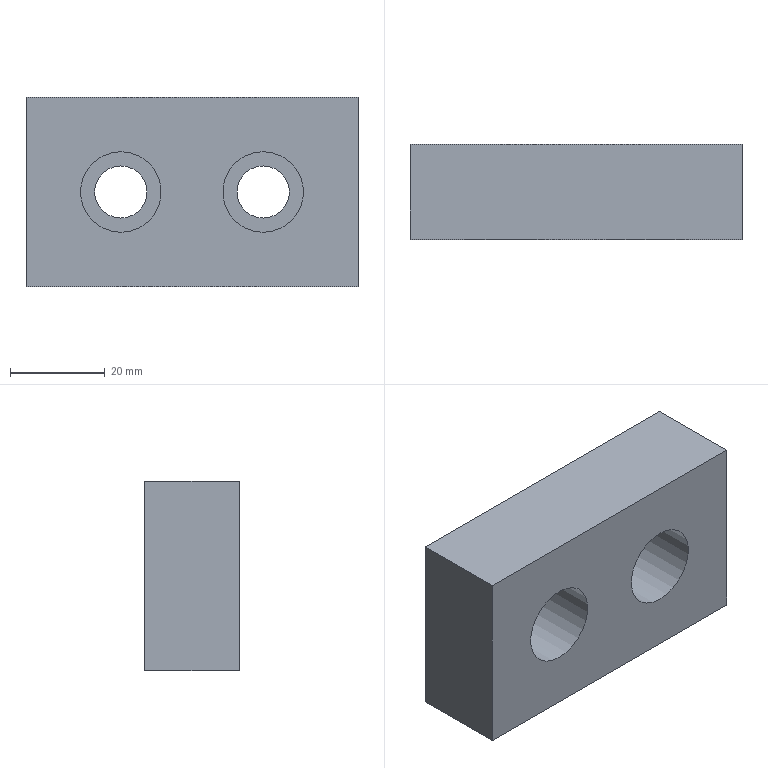Part | NX | features solid 2 | 1 solid | 12 faces | box 70 x 20 x 40 mm | volume 49032 mm3 | plane 8 | cylinder 4 | commonest cylinder face diameters 11 x2 17 x2
STEP:
#1=CARTESIAN_POINT('',(-1202.5,-895.,-295.));
#2=VERTEX_POINT('',#1);
#3=CARTESIAN_POINT('',(-1202.5,-895.,-335.));
#4=VERTEX_POINT('',#3);
#5=CARTESIAN_POINT('',(-1202.5,-895.,-340.));
#6=DIRECTION('',(0.,0.,-1.));
#7=VECTOR('',#6,1000.);
#8=LINE('',#5,#7);
#9=EDGE_CURVE('',#2,#4,#8,.T.);
#10=ORIENTED_EDGE('',*,*,#9,.F.);
#11=CARTESIAN_POINT('',(-1202.5,-875.,-295.));
#12=VERTEX_POINT('',#11);
#13=CARTESIAN_POINT('',(-1202.5,-875.,-295.));
#14=DIRECTION('',(0.,-1.,0.));
#15=VECTOR('',#14,1000.);
#16=LINE('',#13,#15);
#17=EDGE_CURVE('',#12,#2,#16,.T.);
#18=ORIENTED_EDGE('',*,*,#17,.F.);
#19=CARTESIAN_POINT('',(-1202.5,-875.,-335.));
#20=VERTEX_POINT('',#19);
#21=CARTESIAN_POINT('',(-1202.5,-875.,-340.));
#22=DIRECTION('',(0.,0.,-1.));
#23=VECTOR('',#22,1000.);
#24=LINE('',#21,#23);
#25=EDGE_CURVE('',#12,#20,#24,.T.);
#26=ORIENTED_EDGE('',*,*,#25,.T.);
#27=CARTESIAN_POINT('',(-1202.5,-875.,-335.));
#28=DIRECTION('',(0.,-1.,0.));
#29=VECTOR('',#28,1000.);
#30=LINE('',#27,#29);
#31=EDGE_CURVE('',#20,#4,#30,.T.);
#32=ORIENTED_EDGE('',*,*,#31,.T.);
#33=EDGE_LOOP('',(#10,#18,#26,#32));
#34=FACE_BOUND('',#33,.T.);
#35=CARTESIAN_POINT('',(-1202.5,-875.,-340.));
#36=DIRECTION('',(1.,0.,0.));
#37=DIRECTION('',(0.,0.,1.));
#38=AXIS2_PLACEMENT_3D('',#35,#36,#37);
#39=PLANE('',#38);
#40=ADVANCED_FACE('',(#34),#39,.F.);
#41=CARTESIAN_POINT('',(-1132.5,-895.,-295.));
#42=VERTEX_POINT('',#41);
#43=CARTESIAN_POINT('',(77.5,-895.,-295.));
#44=DIRECTION('',(1.,0.,0.));
#45=VECTOR('',#44,1000.);
#46=LINE('',#43,#45);
#47=EDGE_CURVE('',#2,#42,#46,.T.);
#48=ORIENTED_EDGE('',*,*,#47,.T.);
#49=CARTESIAN_POINT('',(-1132.5,-875.,-295.));
#50=VERTEX_POINT('',#49);
#51=CARTESIAN_POINT('',(-1132.5,-875.,-295.));
#52=DIRECTION('',(0.,-1.,0.));
#53=VECTOR('',#52,1000.);
#54=LINE('',#51,#53);
#55=EDGE_CURVE('',#50,#42,#54,.T.);
#56=ORIENTED_EDGE('',*,*,#55,.F.);
#57=CARTESIAN_POINT('',(77.5,-875.,-295.));
#58=DIRECTION('',(1.,0.,0.));
#59=VECTOR('',#58,1000.);
#60=LINE('',#57,#59);
#61=EDGE_CURVE('',#12,#50,#60,.T.);
#62=ORIENTED_EDGE('',*,*,#61,.F.);
#63=ORIENTED_EDGE('',*,*,#17,.T.);
#64=EDGE_LOOP('',(#48,#56,#62,#63));
#65=FACE_BOUND('',#64,.T.);
#66=CARTESIAN_POINT('',(77.5,-875.,-295.));
#67=DIRECTION('',(0.,0.,1.));
#68=DIRECTION('',(-1.,0.,0.));
#69=AXIS2_PLACEMENT_3D('',#66,#67,#68);
#70=PLANE('',#69);
#71=ADVANCED_FACE('',(#65),#70,.T.);
#72=CARTESIAN_POINT('',(-1132.5,-895.,-335.));
#73=VERTEX_POINT('',#72);
#74=CARTESIAN_POINT('',(-1132.5,-895.,-340.));
#75=DIRECTION('',(0.,0.,1.));
#76=VECTOR('',#75,1000.);
#77=LINE('',#74,#76);
#78=EDGE_CURVE('',#73,#42,#77,.T.);
#79=ORIENTED_EDGE('',*,*,#78,.F.);
#80=CARTESIAN_POINT('',(-1132.5,-875.,-335.));
#81=VERTEX_POINT('',#80);
#82=CARTESIAN_POINT('',(-1132.5,-875.,-335.));
#83=DIRECTION('',(0.,-1.,0.));
#84=VECTOR('',#83,1000.);
#85=LINE('',#82,#84);
#86=EDGE_CURVE('',#81,#73,#85,.T.);
#87=ORIENTED_EDGE('',*,*,#86,.F.);
#88=CARTESIAN_POINT('',(-1132.5,-875.,-340.));
#89=DIRECTION('',(0.,0.,1.));
#90=VECTOR('',#89,1000.);
#91=LINE('',#88,#90);
#92=EDGE_CURVE('',#81,#50,#91,.T.);
#93=ORIENTED_EDGE('',*,*,#92,.T.);
#94=ORIENTED_EDGE('',*,*,#55,.T.);
#95=EDGE_LOOP('',(#79,#87,#93,#94));
#96=FACE_BOUND('',#95,.T.);
#97=CARTESIAN_POINT('',(-1132.5,-875.,-340.));
#98=DIRECTION('',(-1.,0.,0.));
#99=DIRECTION('',(0.,0.,-1.));
#100=AXIS2_PLACEMENT_3D('',#97,#98,#99);
#101=PLANE('',#100);
#102=ADVANCED_FACE('',(#96),#101,.F.);
#103=CARTESIAN_POINT('',(77.5,-895.,-335.));
#104=DIRECTION('',(-1.,0.,0.));
#105=VECTOR('',#104,1000.);
#106=LINE('',#103,#105);
#107=EDGE_CURVE('',#73,#4,#106,.T.);
#108=ORIENTED_EDGE('',*,*,#107,.T.);
#109=ORIENTED_EDGE('',*,*,#31,.F.);
#110=CARTESIAN_POINT('',(77.5,-875.,-335.));
#111=DIRECTION('',(-1.,0.,0.));
#112=VECTOR('',#111,1000.);
#113=LINE('',#110,#112);
#114=EDGE_CURVE('',#81,#20,#113,.T.);
#115=ORIENTED_EDGE('',*,*,#114,.F.);
#116=ORIENTED_EDGE('',*,*,#86,.T.);
#117=EDGE_LOOP('',(#108,#109,#115,#116));
#118=FACE_BOUND('',#117,.T.);
#119=CARTESIAN_POINT('',(77.5,-875.,-335.));
#120=DIRECTION('',(0.,0.,-1.));
#121=DIRECTION('',(1.,0.,0.));
#122=AXIS2_PLACEMENT_3D('',#119,#120,#121);
#123=PLANE('',#122);
#124=ADVANCED_FACE('',(#118),#123,.T.);
#125=CARTESIAN_POINT('',(-1182.5,-875.,-309.5));
#126=VERTEX_POINT('',#125);
#127=CARTESIAN_POINT('',(-1182.5,-875.,-315.));
#128=DIRECTION('',(0.,-1.,0.));
#129=DIRECTION('',(0.,0.,1.));
#130=AXIS2_PLACEMENT_3D('',#127,#128,#129);
#131=CIRCLE('',#130,5.5);
#132=EDGE_CURVE('',#126,#126,#131,.T.);
#133=ORIENTED_EDGE('',*,*,#132,.T.);
#134=EDGE_LOOP('',(#133));
#135=FACE_BOUND('',#134,.T.);
#136=CARTESIAN_POINT('',(-1152.5,-875.,-309.5));
#137=VERTEX_POINT('',#136);
#138=CARTESIAN_POINT('',(-1152.5,-875.,-315.));
#139=DIRECTION('',(0.,-1.,0.));
#140=DIRECTION('',(0.,0.,1.));
#141=AXIS2_PLACEMENT_3D('',#138,#139,#140);
#142=CIRCLE('',#141,5.5);
#143=EDGE_CURVE('',#137,#137,#142,.T.);
#144=ORIENTED_EDGE('',*,*,#143,.T.);
#145=EDGE_LOOP('',(#144));
#146=FACE_BOUND('',#145,.T.);
#147=ORIENTED_EDGE('',*,*,#25,.F.);
#148=ORIENTED_EDGE('',*,*,#61,.T.);
#149=ORIENTED_EDGE('',*,*,#92,.F.);
#150=ORIENTED_EDGE('',*,*,#114,.T.);
#151=EDGE_LOOP('',(#147,#148,#149,#150));
#152=FACE_BOUND('',#151,.T.);
#153=CARTESIAN_POINT('',(-1217.5,-875.,-340.));
#154=DIRECTION('',(0.,1.,0.));
#155=DIRECTION('',(1.,0.,0.));
#156=AXIS2_PLACEMENT_3D('',#153,#154,#155);
#157=PLANE('',#156);
#158=ADVANCED_FACE('',(#135,#146,#152),#157,.T.);
#159=CARTESIAN_POINT('',(-1182.5,-895.,-306.5));
#160=VERTEX_POINT('',#159);
#161=CARTESIAN_POINT('',(-1182.5,-895.,-315.));
#162=DIRECTION('',(0.,-1.,0.));
#163=DIRECTION('',(0.,0.,1.));
#164=AXIS2_PLACEMENT_3D('',#161,#162,#163);
#165=CIRCLE('',#164,8.5);
#166=EDGE_CURVE('',#160,#160,#165,.T.);
#167=ORIENTED_EDGE('',*,*,#166,.F.);
#168=EDGE_LOOP('',(#167));
#169=FACE_BOUND('',#168,.T.);
#170=CARTESIAN_POINT('',(-1152.5,-895.,-306.5));
#171=VERTEX_POINT('',#170);
#172=CARTESIAN_POINT('',(-1152.5,-895.,-315.));
#173=DIRECTION('',(0.,-1.,0.));
#174=DIRECTION('',(0.,0.,1.));
#175=AXIS2_PLACEMENT_3D('',#172,#173,#174);
#176=CIRCLE('',#175,8.5);
#177=EDGE_CURVE('',#171,#171,#176,.T.);
#178=ORIENTED_EDGE('',*,*,#177,.F.);
#179=EDGE_LOOP('',(#178));
#180=FACE_BOUND('',#179,.T.);
#181=ORIENTED_EDGE('',*,*,#9,.T.);
#182=ORIENTED_EDGE('',*,*,#107,.F.);
#183=ORIENTED_EDGE('',*,*,#78,.T.);
#184=ORIENTED_EDGE('',*,*,#47,.F.);
#185=EDGE_LOOP('',(#181,#182,#183,#184));
#186=FACE_BOUND('',#185,.T.);
#187=CARTESIAN_POINT('',(-1217.5,-895.,-340.));
#188=DIRECTION('',(0.,1.,0.));
#189=DIRECTION('',(1.,0.,0.));
#190=AXIS2_PLACEMENT_3D('',#187,#188,#189);
#191=PLANE('',#190);
#192=ADVANCED_FACE('',(#169,#180,#186),#191,.F.);
#193=ORIENTED_EDGE('',*,*,#143,.F.);
#194=EDGE_LOOP('',(#193));
#195=FACE_BOUND('',#194,.T.);
#196=CARTESIAN_POINT('',(-1152.5,-883.,-309.5));
#197=VERTEX_POINT('',#196);
#198=CARTESIAN_POINT('',(-1152.5,-883.,-315.));
#199=DIRECTION('',(0.,-1.,0.));
#200=DIRECTION('',(0.,0.,1.));
#201=AXIS2_PLACEMENT_3D('',#198,#199,#200);
#202=CIRCLE('',#201,5.5);
#203=EDGE_CURVE('',#197,#197,#202,.T.);
#204=ORIENTED_EDGE('',*,*,#203,.T.);
#205=EDGE_LOOP('',(#204));
#206=FACE_BOUND('',#205,.T.);
#207=CARTESIAN_POINT('',(-1152.5,-845.,-315.));
#208=DIRECTION('',(0.,1.,0.));
#209=DIRECTION('',(0.,0.,1.));
#210=AXIS2_PLACEMENT_3D('',#207,#208,#209);
#211=CYLINDRICAL_SURFACE('',#210,5.5);
#212=ADVANCED_FACE('',(#195,#206),#211,.F.);
#213=ORIENTED_EDGE('',*,*,#203,.F.);
#214=EDGE_LOOP('',(#213));
#215=FACE_BOUND('',#214,.T.);
#216=CARTESIAN_POINT('',(-1152.5,-883.,-306.5));
#217=VERTEX_POINT('',#216);
#218=CARTESIAN_POINT('',(-1152.5,-883.,-315.));
#219=DIRECTION('',(0.,-1.,0.));
#220=DIRECTION('',(0.,0.,1.));
#221=AXIS2_PLACEMENT_3D('',#218,#219,#220);
#222=CIRCLE('',#221,8.5);
#223=EDGE_CURVE('',#217,#217,#222,.T.);
#224=ORIENTED_EDGE('',*,*,#223,.T.);
#225=EDGE_LOOP('',(#224));
#226=FACE_BOUND('',#225,.T.);
#227=CARTESIAN_POINT('',(-1152.5,-883.,-315.));
#228=DIRECTION('',(0.,1.,0.));
#229=DIRECTION('',(0.,0.,1.));
#230=AXIS2_PLACEMENT_3D('',#227,#228,#229);
#231=PLANE('',#230);
#232=ADVANCED_FACE('',(#215,#226),#231,.F.);
#233=ORIENTED_EDGE('',*,*,#223,.F.);
#234=EDGE_LOOP('',(#233));
#235=FACE_BOUND('',#234,.T.);
#236=ORIENTED_EDGE('',*,*,#177,.T.);
#237=EDGE_LOOP('',(#236));
#238=FACE_BOUND('',#237,.T.);
#239=CARTESIAN_POINT('',(-1152.5,-895.,-315.));
#240=DIRECTION('',(0.,1.,0.));
#241=DIRECTION('',(0.,0.,1.));
#242=AXIS2_PLACEMENT_3D('',#239,#240,#241);
#243=CYLINDRICAL_SURFACE('',#242,8.5);
#244=ADVANCED_FACE('',(#235,#238),#243,.F.);
#245=ORIENTED_EDGE('',*,*,#132,.F.);
#246=EDGE_LOOP('',(#245));
#247=FACE_BOUND('',#246,.T.);
#248=CARTESIAN_POINT('',(-1182.5,-883.,-309.5));
#249=VERTEX_POINT('',#248);
#250=CARTESIAN_POINT('',(-1182.5,-883.,-315.));
#251=DIRECTION('',(0.,-1.,0.));
#252=DIRECTION('',(0.,0.,1.));
#253=AXIS2_PLACEMENT_3D('',#250,#251,#252);
#254=CIRCLE('',#253,5.5);
#255=EDGE_CURVE('',#249,#249,#254,.T.);
#256=ORIENTED_EDGE('',*,*,#255,.T.);
#257=EDGE_LOOP('',(#256));
#258=FACE_BOUND('',#257,.T.);
#259=CARTESIAN_POINT('',(-1182.5,-845.,-315.));
#260=DIRECTION('',(0.,1.,0.));
#261=DIRECTION('',(0.,0.,1.));
#262=AXIS2_PLACEMENT_3D('',#259,#260,#261);
#263=CYLINDRICAL_SURFACE('',#262,5.5);
#264=ADVANCED_FACE('',(#247,#258),#263,.F.);
#265=ORIENTED_EDGE('',*,*,#255,.F.);
#266=EDGE_LOOP('',(#265));
#267=FACE_BOUND('',#266,.T.);
#268=CARTESIAN_POINT('',(-1182.5,-883.,-306.5));
#269=VERTEX_POINT('',#268);
#270=CARTESIAN_POINT('',(-1182.5,-883.,-315.));
#271=DIRECTION('',(0.,-1.,0.));
#272=DIRECTION('',(0.,0.,1.));
#273=AXIS2_PLACEMENT_3D('',#270,#271,#272);
#274=CIRCLE('',#273,8.5);
#275=EDGE_CURVE('',#269,#269,#274,.T.);
#276=ORIENTED_EDGE('',*,*,#275,.T.);
#277=EDGE_LOOP('',(#276));
#278=FACE_BOUND('',#277,.T.);
#279=CARTESIAN_POINT('',(-1182.5,-883.,-315.));
#280=DIRECTION('',(0.,1.,0.));
#281=DIRECTION('',(0.,0.,1.));
#282=AXIS2_PLACEMENT_3D('',#279,#280,#281);
#283=PLANE('',#282);
#284=ADVANCED_FACE('',(#267,#278),#283,.F.);
#285=ORIENTED_EDGE('',*,*,#275,.F.);
#286=EDGE_LOOP('',(#285));
#287=FACE_BOUND('',#286,.T.);
#288=ORIENTED_EDGE('',*,*,#166,.T.);
#289=EDGE_LOOP('',(#288));
#290=FACE_BOUND('',#289,.T.);
#291=CARTESIAN_POINT('',(-1182.5,-895.,-315.));
#292=DIRECTION('',(0.,1.,0.));
#293=DIRECTION('',(0.,0.,1.));
#294=AXIS2_PLACEMENT_3D('',#291,#292,#293);
#295=CYLINDRICAL_SURFACE('',#294,8.5);
#296=ADVANCED_FACE('',(#287,#290),#295,.F.);
#297=CLOSED_SHELL('',(#40,#71,#102,#124,#158,#192,#212,#232,#244,#264,#284,#296));
#298=MANIFOLD_SOLID_BREP('',#297);
#299=(LENGTH_UNIT()NAMED_UNIT(*)SI_UNIT(.MILLI.,.METRE.));
#300=UNCERTAINTY_MEASURE_WITH_UNIT(LENGTH_MEASURE(0.00001),#299,'','');
#301=(NAMED_UNIT(*)PLANE_ANGLE_UNIT()SI_UNIT($,.RADIAN.));
#302=(NAMED_UNIT(*)SI_UNIT($,.STERADIAN.)SOLID_ANGLE_UNIT());
#303=(GEOMETRIC_REPRESENTATION_CONTEXT(3)GLOBAL_UNCERTAINTY_ASSIGNED_CONTEXT((#300))GLOBAL_UNIT_ASSIGNED_CONTEXT((#299,#301,#302))REPRESENTATION_CONTEXT('',''));
#304=ADVANCED_BREP_SHAPE_REPRESENTATION('',(#298),#303);